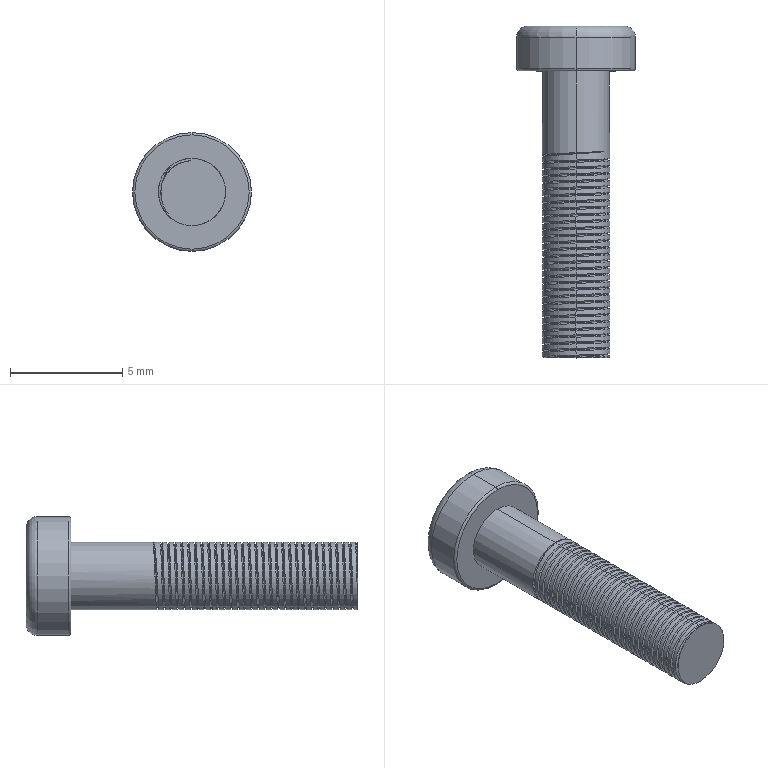Part | SolidWorks | features Fillet 2, Helix 2, ICE 2, SweepCut 2, Extrusion 1 | 1 solid | 92 faces | box 5.3 x 14.8 x 5.3 mm | volume 130.333 mm3 | cylinder 65 | plane 17 | spline 6 | torus 4 | commonest cylinder face diameters 3 x63 5.3 x2